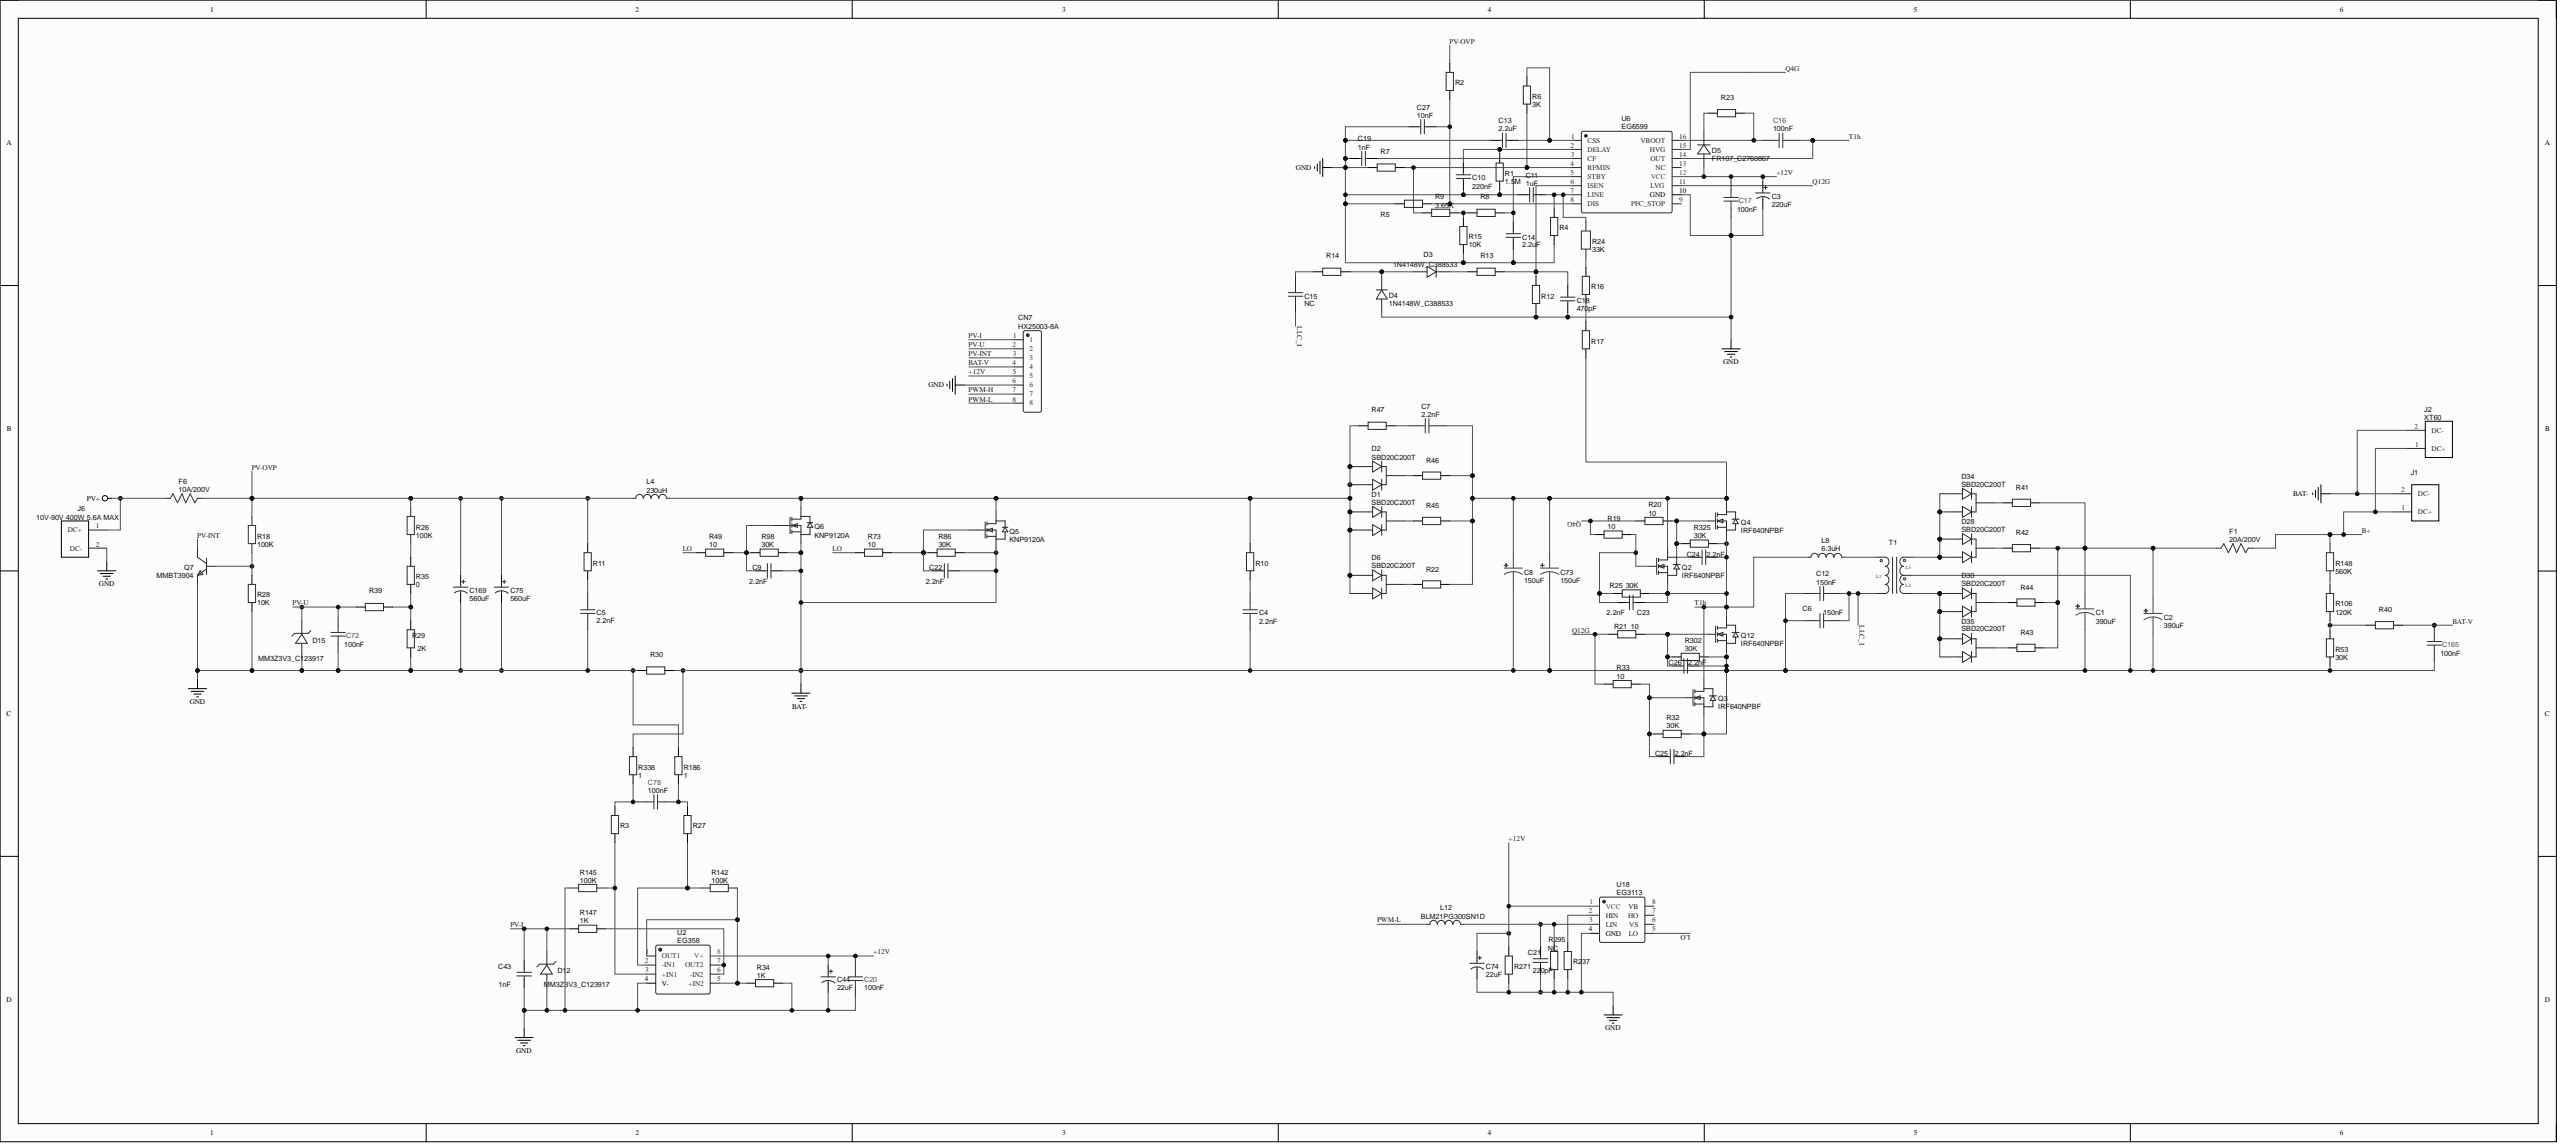Circuit board | Altium Designer | 128 parts | 67 nets
Bill of materials:
Comment,Description,Designator,Footprint,LibRef,Quantity
"390uF","","C1, C2","CAP-TH_BD10.0-P5.00-D1.0-FD","390uF","2"
"220uF","","C3","CAP-TH_BD6.3-P2.50-D1.0-FD","220uF","1"
"2.2nF","","C4, C5, C7","C1206","2.2nF","3"
"150nF","","C6, C12","CAP-TH_L17.0-W6.5-P15.00-D1.2","150nF","2"
"150uF","","C8, C73","CAP-TH_BD12.5-P5.00-D0.6-FD","150uF","2"
"2.2nF","","C9, C22, C23, C24, C25, C26","C0603","2.2nF","6"
"220nF","","C10","C0603","220nF","1"
"1uF","","C11","C0603","1uF","1"
"2.2uF","","C13, C14","C0603","2.2uF","2"
"NC","","C15","C1206","NC","1"
"100nF","","C16, C17, C20, C72, C78, C165","C0603","100nF","6"
"470pF","","C18","C0603","470pF","1"
"1nF","","C19, C43","C0603","1nF","2"
"220pF","","C21","C0603","220pF","1"
"10nF","","C27","C1206","10nF","1"
"22uF","","C44, C74","CAP-TH_BD5.0-P2.00-D0.8-FD","22uF","2"
"560uF","","C75, C169","CAP-TH_BD16.0-P7.50-D1.2-FD","560uF","2"
"HX25003-8A","","CN7","CONN-TH_8P-P2.50_HX25003-8A","HX25003-8A","1"
"SBD20C200T","","D1, D2, D6","TO-220-3_L10.0-W4.5-P2.54-L","SBD20C200T","3"
"1N4148W_C388533","","D3, D4","SOD-123_L2.8-W1.8-LS3.7-RD","1N4148W_C388533","2"
"FR107_C2760867","","D5","SOD-123FL_L2.7-W1.8-LS3.8-RD","FR107_C2760867","1"
"MM3Z3V3_C123917","","D12, D15","SOD-323_L1.8-W1.3-LS2.5-RD","MM3Z3V3_C123917","2"
"SBD20C200T","","D28, D30, D34, D35","TO-220-3_L10.0-W4.5-P2.54-L-N","SBD20C200T","4"
"20A/200V","","F1","FUSE-SMD_L6.1-W2.5","20A/200V","1"
"10A/200V","","F6","FUSE-SMD_L6.1-W2.5","10A/200V","1"
"","","J1","XT90N","","1"
"XT60","","J2","CONN-TH_XT60UPB-F","XT60","1"
"10V-90V 400W 5.6A MAX","","J6","XT90","10V-90V 400W 5.6A MAX","1"
"230uH","","L4","IND-TH_CS343090*2-W231K","230uH","1"
"6.3uH","","L8","PQ2620-N","6.3uH","1"
"BLM21PG300SN1D","","L12","L0805","BLM21PG300SN1D","1"
"IRF640NPBF","","Q2, Q3, Q4, Q12","TO-220-3_L10.0-W4.5-P2.54-L-N","IRF640NPBF","4"
"KNP9120A","","Q5, Q6","TO-220-3_L10.0-W4.5-P2.54-L","KNP9120A","2"
"MMBT3904","","Q7","SOT-23-3_L2.9-W1.3-P1.90-LS2.4-BR","MMBT3904","1"
"1.5M","","R1","R0603","1.5M","1"
"","","R2, R5, R23","R0805","","3"
"","","R3, R4, R7, R8, R12, R13, R14, R27, R39, R40, R237, R271","R0603","","12"
"3K","","R6","R0603","3K","1"
"3.65K","","R9","R0603","3.65K","1"
"","","R10, R11, R16, R17, R47","R1206","","5"
"10K","","R15, R28","R1206","10K","2"
"100K","","R18, R26, R142, R145","R0805","100K","4"
"10","","R19, R20, R21, R33, R49, R73","R1206","10","6"
"","","R22, R30, R41, R42, R43, R44, R45, R46","R2512","","8"
"33K","","R24","R1206","33K","1"
"30K","","R25, R32, R53, R86, R98, R302, R325","R0603","30K","7"
"2K","","R29","R0603","2K","1"
"1K","","R34, R147","R0603","1K","2"
"0","","R35","R0805","0","1"
"120K","","R106","R0603","120K","1"
"560K","","R148","R0603","560K","1"
"1","","R186, R338","R0603","1","2"
"NC","","R295","R0603","NC","1"
"","","T1","PQ3230 3:2:2-N","","1"
"EG358","","U2","SOIC-8_L5.0-W4.0-P1.27-LS6.0-BL","EG358","1"
"EG6599","","U6","SO-16_L10.0-W4.0-P1.27-LS6.2-BL","EG6599","1"
"EG3113","","U18","SOP-8_L4.9-W3.9-P1.27-LS6.0-BL","EG3113","1"
Netlist (Protel format):
[
C1
CAP-TH_BD10.0-P5.00-D1.0-FD
390uF



]
[
C2
CAP-TH_BD10.0-P5.00-D1.0-FD
390uF



]
[
C3
CAP-TH_BD6.3-P2.50-D1.0-FD
220uF



]
[
C4
C1206
2.2nF



]
[
C5
C1206
2.2nF



]
[
C6
CAP-TH_L17.0-W6.5-P15.00-D1.2
150nF



]
[
C7
C1206
2.2nF



]
[
C8
CAP-TH_BD12.5-P5.00-D0.6-FD
150uF



]
[
C9
C0603
2.2nF



]
[
C10
C0603
220nF



]
[
C11
C0603
1uF



]
[
C12
CAP-TH_L17.0-W6.5-P15.00-D1.2
150nF



]
[
C13
C0603
2.2uF



]
[
C14
C0603
2.2uF



]
[
C15
C1206
NC



]
[
C16
C0603
100nF



]
[
C17
C0603
100nF



]
[
C18
C0603
470pF



]
[
C19
C0603
1nF



]
[
C20
C0603
100nF



]
[
C21
C0603
220pF



]
[
C22
C0603
2.2nF



]
[
C23
C0603
2.2nF



]
[
C24
C0603
2.2nF



]
[
C25
C0603
2.2nF



]
[
C26
C0603
2.2nF



]
[
C27
C1206
10nF



]
[
C43
C0603
1nF



]
[
C44
CAP-TH_BD5.0-P2.00-D0.8-FD
22uF



]
[
C72
C0603
100nF



]
[
C73
CAP-TH_BD12.5-P5.00-D0.6-FD
150uF



]
[
C74
CAP-TH_BD5.0-P2.00-D0.8-FD
22uF



]
[
C75
CAP-TH_BD16.0-P7.50-D1.2-FD
560uF



]
[
C78
C0603
100nF



]
[
C165
C0603
100nF



]
[
C169
CAP-TH_BD16.0-P7.50-D1.2-FD
560uF



]
[
CN7
CONN-TH_8P-P2.50_HX25003-8A
HX25003-8A



]
[
D1
TO-220-3_L10.0-W4.5-P2.54-L
SBD20C200T



]
[
D2
TO-220-3_L10.0-W4.5-P2.54-L
SBD20C200T



]
[
D3
SOD-123_L2.8-W1.8-LS3.7-RD
1N4148W_C388533



]
[
D4
SOD-123_L2.8-W1.8-LS3.7-RD
1N4148W_C388533



]
[
D5
SOD-123FL_L2.7-W1.8-LS3.8-RD
FR107_C2760867



]
[
D6
TO-220-3_L10.0-W4.5-P2.54-L
SBD20C200T



]
[
D12
SOD-323_L1.8-W1.3-LS2.5-RD
MM3Z3V3_C123917



]
[
D15
SOD-323_L1.8-W1.3-LS2.5-RD
MM3Z3V3_C123917



]
[
D28
TO-220-3_L10.0-W4.5-P2.54-L-N
SBD20C200T



]
[
D30
TO-220-3_L10.0-W4.5-P2.54-L-N
SBD20C200T



]
[
D34
TO-220-3_L10.0-W4.5-P2.54-L-N
SBD20C200T



]
[
D35
TO-220-3_L10.0-W4.5-P2.54-L-N
SBD20C200T



]
[
F1
FUSE-SMD_L6.1-W2.5
20A/200V



]
[
F6
FUSE-SMD_L6.1-W2.5
10A/200V



]
[
J1
XT90N




]
[
J2
CONN-TH_XT60UPB-F
XT60



]
[
J6
XT90
10V-90V 400W 5.6A MAX



]
[
L4
IND-TH_CS343090*2-W231K
230uH



]
[
L8
PQ2620-N
6.3uH



]
[
L12
L0805
BLM21PG300SN1D



]
[
Q2
TO-220-3_L10.0-W4.5-P2.54-L-N
IRF640NPBF



]
[
Q3
TO-220-3_L10.0-W4.5-P2.54-L-N
IRF640NPBF



]
[
Q4
TO-220-3_L10.0-W4.5-P2.54-L-N
IRF640NPBF



]
[
Q5
TO-220-3_L10.0-W4.5-P2.54-L
KNP9120A



]
[
Q6
TO-220-3_L10.0-W4.5-P2.54-L
KNP9120A



]
[
Q7
SOT-23-3_L2.9-W1.3-P1.90-LS2.4-BR
MMBT3904



]
[
Q12
TO-220-3_L10.0-W4.5-P2.54-L-N
IRF640NPBF



]
[
R1
R0603
1.5M



]
[
R2
R0805




]
[
R3
R0603




]
[
R4
R0603




]
[
R5
R0805




]
[
R6
R0603
3K



]
[
R7
R0603




]
[
R8
R0603




]
[
R9
R0603
3.65K



]
[
R10
R1206




]
[
R11
R1206




]
[
R12
R0603




]
[
R13
R0603




]
[
R14
R0603




]
[
R15
R1206
10K



]
[
R16
R1206




]
[
R17
R1206




]
[
R18
R0805
100K



]
[
R19
R1206
10



]
[
R20
R1206
10



]
[
R21
R1206
10



]
[
R22
R2512




]
[
R23
R0805




]
[
R24
R1206
33K



]
[
R25
R0603
30K



]
[
R26
R0805
100K



]
[
R27
R0603




]
[
R28
R1206
10K



]
[
R29
R0603
2K



]
[
R30
R2512




]
[
R32
R0603
30K



]
[
R33
R1206
10



]
[
R34
R0603
1K



]
[
R35
R0805
0



]
[
R39
R0603




]
[
R40
R0603




]
[
R41
R2512




]
[
R42
R2512




]
[
R43
R2512




]
[
R44
R2512




]
[
R45
R2512




]
[
R46
R2512




]
[
R47
R1206




]
[
R49
R1206
10



]
[
R53
R0603
30K



]
[
R73
R1206
10



]
[
R86
R0603
30K



]
[
R98
R0603
30K



]
[
R106
R0603
120K



]
[
R142
R0805
100K



]
[
R145
R0805
100K



]
[
R147
R0603
1K



]
[
R148
R0603
560K



]
[
R186
R0603
1



]
[
R237
R0603




]
[
R271
R0603




]
[
R295
R0603
NC



]
[
R302
R0603
30K



]
[
R325
R0603
30K



]
[
R338
R0603
1



]
[
T1
PQ3230 3:2:2-N




]
[
U2
SOIC-8_L5.0-W4.0-P1.27-LS6.0-BL
EG358



]
[
U6
SO-16_L10.0-W4.0-P1.27-LS6.2-BL
EG6599



]
[
U18
SOP-8_L4.9-W3.9-P1.27-LS6.0-BL
EG3113



]
(
T1h
C16-1
C23-2
C24-2
L8-3
Q2-3
Q3-2
Q4-3
Q12-2
R25-2
R325-2
U6-14
)
(
Q12G
R21-1
R33-1
U6-11
)
(
Q4G
R19-1
R20-1
U6-15
)
(
PWM-L
CN7-8
L12-1
)
(
PV-U
C72-2
CN7-2
D15-1
R39-2
)
(
PV-OVP
C75-1
C169-1
F6-2
L4-1
R2-2
R11-1
R18-2
R26-2
)
(
PV-INT
CN7-3
Q7-3
)
(
PV-I
C43-2
CN7-1
D12-1
R147-2
)
(
PV+
F6-1
J6-1
)
(
NetR237_2
R237-2
U18-2
)
(
NetR147_1
R147-1
U2-6
U2-7
)
(
NetR106_2
R106-2
R148-1
)
(
NetR40_2
R40-2
R53-2
R106-1
)
(
NetR34_1
R34-1
R142-1
U2-1
U2-5
)
(
NetR29_1
R29-1
R35-1
R39-1
)
(
NetR27_1
R27-1
R142-2
U2-2
)
(
NetR26_1
R26-1
R35-2
)
(
NetR16_2
R16-2
R24-1
)
(
NetR16_1
R16-1
R17-2
)
(
NetR8_1
R8-1
R9-2
R15-1
)
(
NetR6_1
R6-1
R7-1
R9-1
U6-4
)
(
NetR3_1
R3-1
R145-1
U2-3
)
(
NetQ7_1
Q7-1
R18-1
R28-1
)
(
NetL8_4
L8-4
T1-4
)
(
NetD35_2
D35-2
R43-1
)
(
NetD34_2
D34-2
R41-1
)
(
NetD30_2
D30-2
R44-1
)
(
NetD30_1
D30-1
D30-3
D35-1
D35-3
T1-10
)
(
NetD28_2
D28-2
R42-1
)
(
NetD28_1
D28-1
D28-3
D34-1
D34-3
T1-8
)
(
NetD6_2
D6-2
R22-1
)
(
NetD5_1
D5-1
R23-2
)
(
NetD3_2
D3-2
D4-1
R14-2
)
(
NetD3_1
D3-1
R13-1
)
(
NetD2_2
D2-2
R46-1
)
(
NetD1_2
D1-2
R45-1
)
(
NetD1_1
D1-1
D1-3
D2-1
D2-3
D6-1
D6-3
L4-2
Q5-2
Q6-2
R10-1
R47-1
)
(
NetC78_2
C78-2
R3-2
R338-1
)
(
NetC78_1
C78-1
R27-2
R186-1
)
(
NetC27_2
C27-2
R2-1
R5-2
U6-8
)
(
NetC26_1
C26-1
Q12-1
R21-2
R302-1
)
(
NetC25_1
C25-1
Q3-1
R32-1
R33-2
)
(
NetC24_1
C24-1
Q4-1
R20-2
R325-1
)
(
NetC23_1
C23-1
Q2-1
R19-2
R25-1
)
(
NetC22_1
C22-1
Q5-1
R73-2
R86-2
)
(
NetC21_2
C21-2
L12-2
R295-1
U18-3
)
(
NetC19_1
C19-1
U6-3
)
(
NetC18_2
C18-2
R12-2
R13-2
U6-6
)
(
NetC16_2
C16-2
R23-1
U6-16
)
(
NetC15_2
C15-2
R14-1
)
(
NetC14_2
C14-2
R8-2
U6-5
)
(
NetC13_2
C13-2
R6-2
U6-1
)
(
NetC11_1
C11-1
R4-2
R24-2
U6-7
)
(
NetC10_2
C10-2
R1-2
U6-2
)
(
NetC9_1
C9-1
Q6-1
R49-2
R98-2
)
(
NetC7_2
C7-2
C8-1
C73-1
Q2-2
Q4-2
R17-1
R22-2
R45-2
R46-2
)
(
NetC7_1
C7-1
R47-2
)
(
NetC5_1
C5-1
R11-2
)
(
NetC4_1
C4-1
R10-2
)
(
NetC1_1
C1-1
C2-1
F1-1
R41-2
R42-2
R43-2
R44-2
)
(
LO
R49-1
R73-1
U18-5
)
(
LLC_I
C6-1
C12-1
C15-1
T1-3
)
(
GND
C3-2
C5-2
C10-1
C11-2
C13-1
C14-1
C17-1
C18-1
C19-2
C20-2
C21-1
C27-1
C43-1
C44-2
C72-1
C74-2
C75-2
C169-2
CN7-6
D4-2
D12-2
D15-2
J6-2
Q7-2
R1-1
R4-1
R5-1
R7-2
R12-1
R15-2
R28-2
R29-2
R30-1
R34-2
R145-2
R186-2
R237-1
R271-1
R295-2
U2-4
U6-10
U18-4
)
(
BAT-V
C165-2
CN7-4
R40-1
)
(
BAT-
C1-2
C2-2
C4-2
C6-2
C8-2
C9-2
C12-2
C22-2
C25-2
C26-2
C73-2
C165-1
J1-2
J2-2
Q3-3
Q5-3
Q6-3
Q12-3
R30-2
R32-2
R53-1
R86-1
R98-1
R302-2
R338-2
T1-9
)
(
B+
F1-2
J1-1
J2-1
R148-2
)
(
+12V
C3-1
C17-2
C20-1
C44-1
C74-1
CN7-5
D5-2
R271-2
U2-8
U6-12
U18-1
)